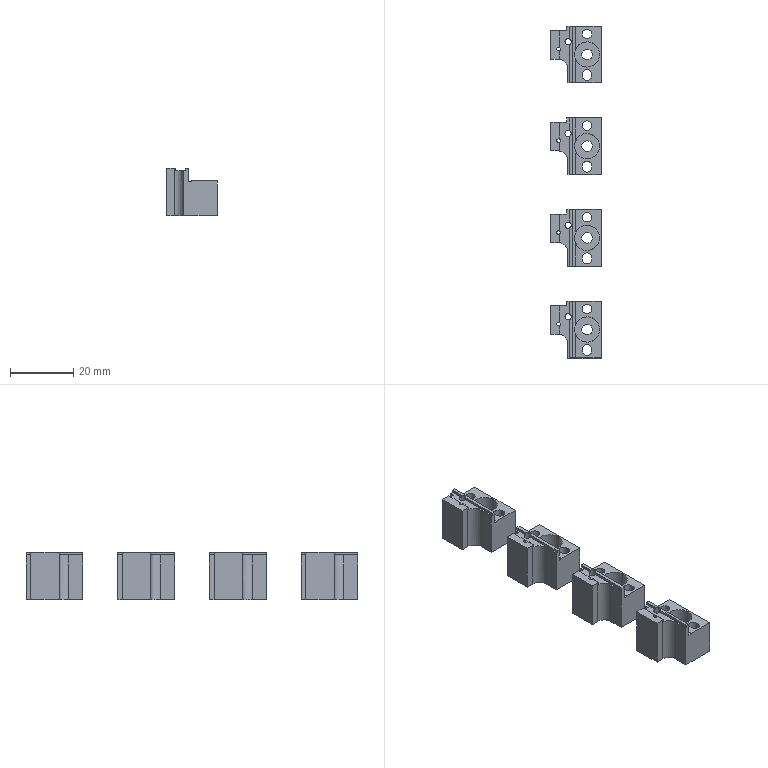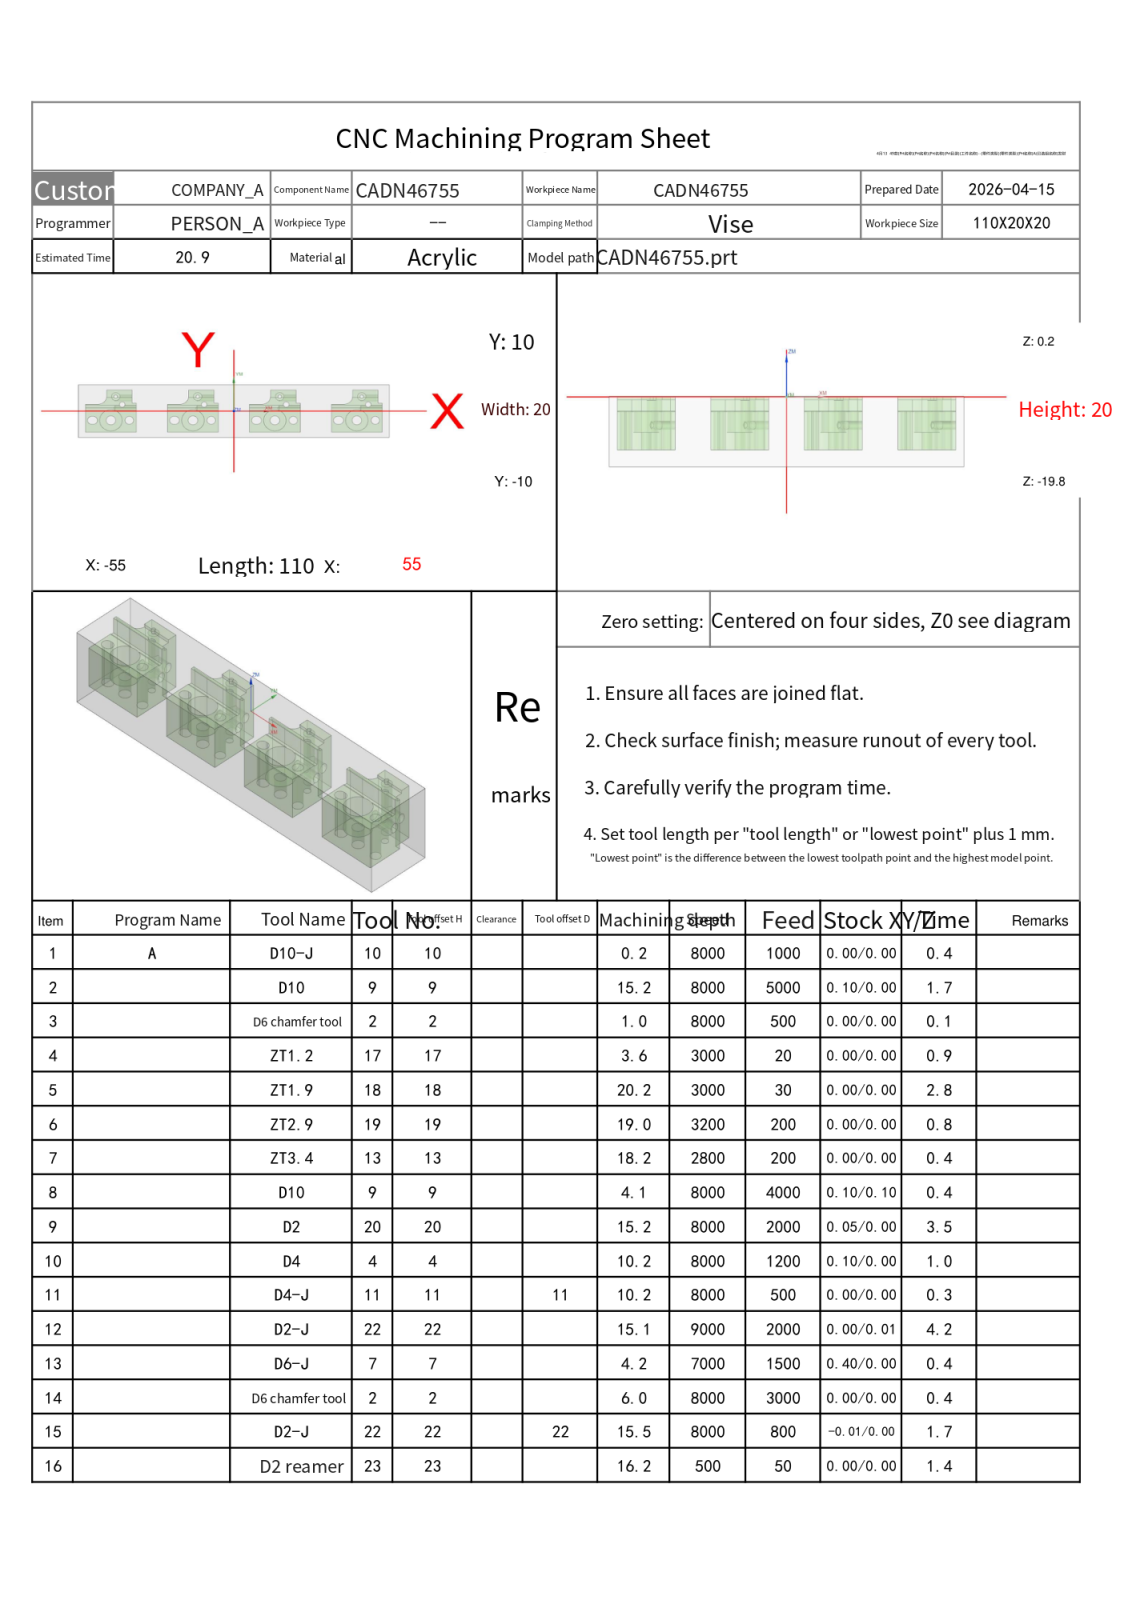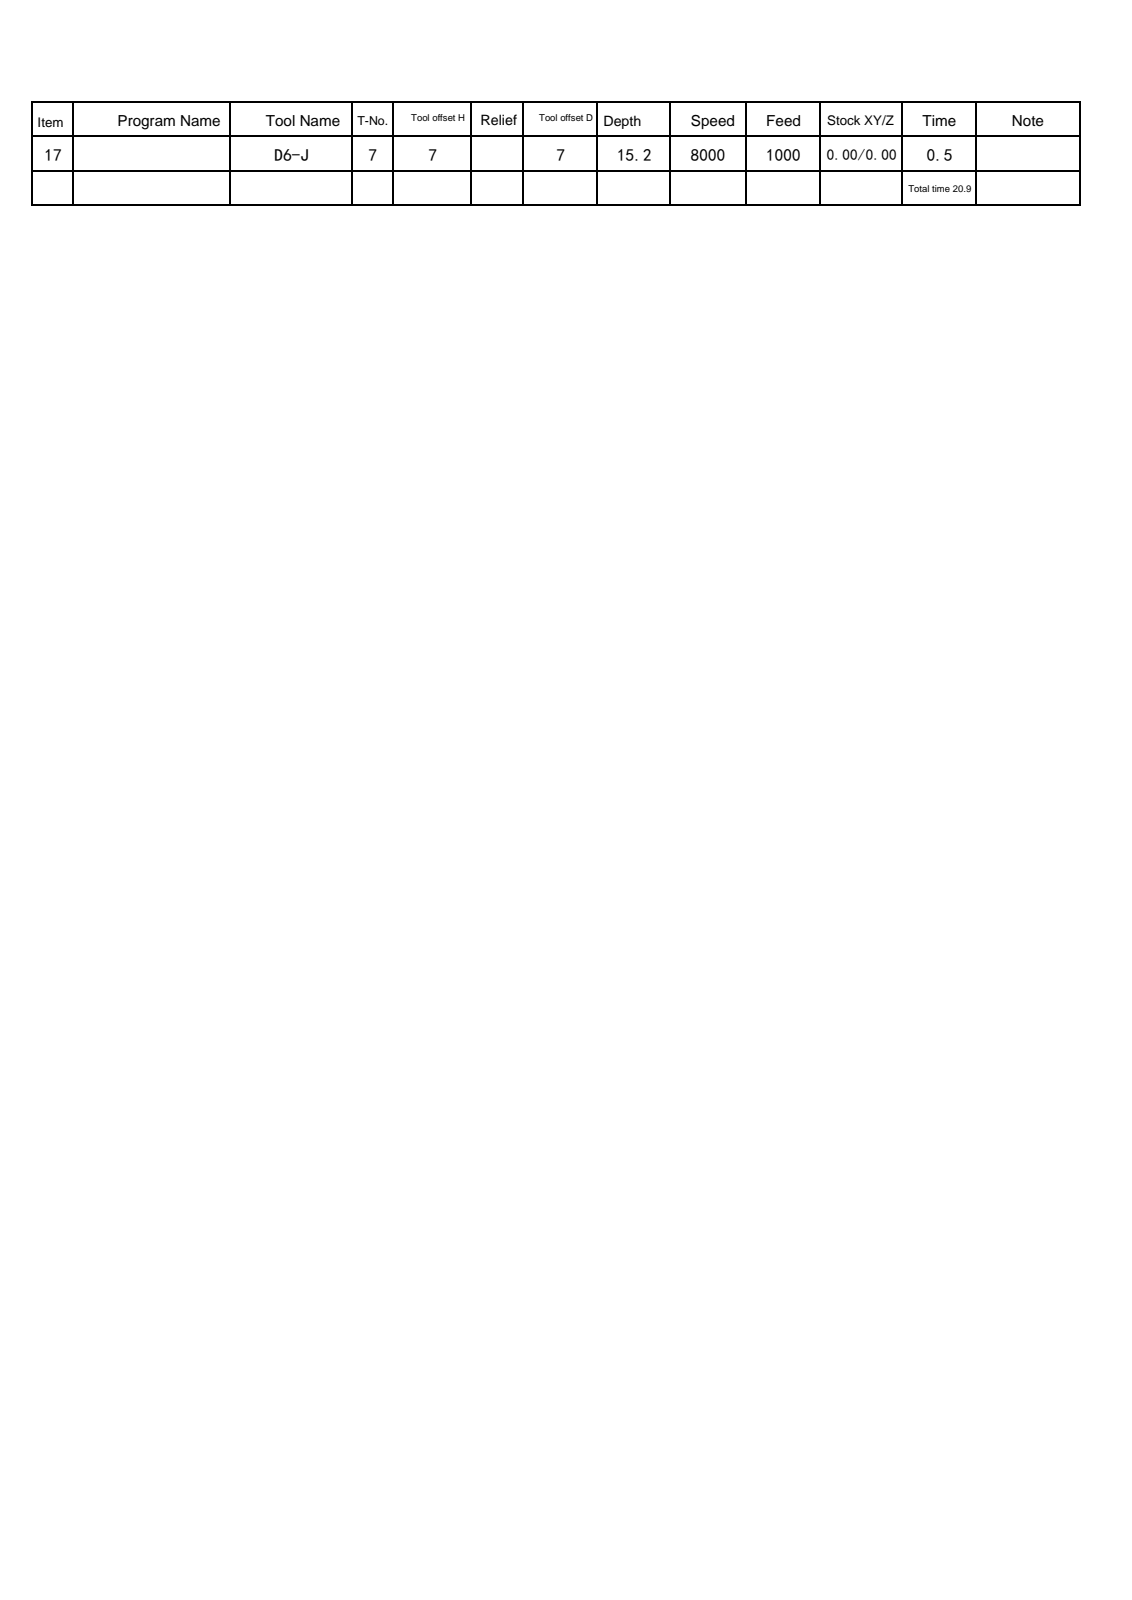NC program | NX | posted by the shop | part box 16 x 105 x 15 mm
Lines 1 to 1402 of 25120, first 1314 of 1400 lines:
%
O0001
(Machine time: 24.18 MIN)
(===Total Tool:13===)
(T10=D10-J  D=10.  R=0.   D-  H10 Z=-0.   )
(T9=D10     D=10.  R=0.   D-  H09 Z=-15.  )
(T2=D6 chamfer tool   D=6.   R=0.   D-  H02 Z=-5.8  )
(T17=ZT1.2  D=1.2  DR_a=118 D-  H17 Z=-3.36 )
(T18=ZT1.9  D=1.9  DR_a=120 D-  H18 Z=-20.  )
(T19=ZT2.9  D=2.9  DR_a=120 D-  H19 Z=-18.84)
(T13=ZT3.4  D=3.4  DR_a=118 D-  H13 Z=-18.02)
(T20=D2     D=2.   R=0.   D-  H20 Z=-15.  )
(T4=D4      D=4.   R=0.   D-  H04 Z=-10.  )
(T11=D4-J   D=4.   R=0.   D11 H11 Z=-10.  )
(T22=D2-J   D=2.   R=0.   D-  H22 Z=-15.3 )
(T7=D6-J    D=6.   R=0.   D-  H07 Z=-15.  )
(T23=D2 reamer   D=1.95 DR_a=180 D23 H23 Z=-16.  )
G80 G90 G17 G49 G40
G91 G28 Z0
M01
N1 T10 M06
(D10-J  D=10. R=0. H=10 ce=0.00 di=0.00)
G00 G90 G54 X-62.5 Y6.5 M03 S8000
G43 H10 Z20.
M08
Z2.
G01 Z0.0 F1000.
X-57.5
X57.5
Y0.0
X-57.5
Y-6.5
X57.5
X62.5
Z2.
G00 Z20.
G91 G28 Z0.0
M05
M09
G91 G28 Z0.0
M01
N2 T09 M06
(D10  D=10. R=0. H=09 ce=0.10 di=0.00)
G00 G90 G54 X43.5 Y-13.1 M03 S8000
G43 H09 Z20.
M08
Z.5
G01 X34.5 Z.428 F5000.
G02 X29.4 Y-8. Z.364 I0.0 J5.1
G01 Y2.6 Z.279
G02 X34.5 Y7.7 Z.215 I5.1 J0.0
G01 X36.9 Z.195
Y8. Z.193
G02 X42. Y13.1 Z.129 I5.1 J0.0
G01 X51. Z.057
G02 X56.1 Y8. Z-.007 I0.0 J-5.1
G01 Y6.612 Z-.018
G02 X57.6 Y3. Z-.051 I-3.6 J-3.612
G01 Y-8. Z-.139
G02 X52.5 Y-13.1 Z-.203 I-5.1 J0.0
G01 X34.5 Z-.347
G02 X29.4 Y-8. Z-.411 I0.0 J5.1
G01 Y2.6 Z-.496
G02 X34.5 Y7.7 Z-.56 I5.1 J0.0
G01 X36.9 Z-.58
Y8. Z-.582
G02 X42. Y13.1 Z-.646 I5.1 J0.0
G01 X51. Z-.718
G02 X56.1 Y8. Z-.782 I0.0 J-5.1
G01 Y6.612 Z-.793
G02 X57.6 Y3. Z-.826 I-3.6 J-3.612
G01 Y-8. Z-.914
G02 X52.5 Y-13.1 Z-.978 I-5.1 J0.0
G01 X34.5 Z-1.122
G02 X29.4 Y-8. Z-1.186 I0.0 J5.1
G01 Y2.6 Z-1.271
G02 X34.5 Y7.7 Z-1.335 I5.1 J0.0
G01 X36.9 Z-1.355
Y8. Z-1.357
G02 X42. Y13.1 Z-1.421 I5.1 J0.0
G01 X51. Z-1.493
G02 X56.1 Y8. Z-1.557 I0.0 J-5.1
G01 Y6.612 Z-1.568
G02 X57.6 Y3. Z-1.601 I-3.6 J-3.612
G01 Y-8. Z-1.689
G02 X52.5 Y-13.1 Z-1.753 I-5.1 J0.0
G01 X34.5 Z-1.897
G02 X29.4 Y-8. Z-1.961 I0.0 J5.1
G01 Y2.6 Z-2.046
G02 X34.5 Y7.7 Z-2.11 I5.1 J0.0
G01 X36.9 Z-2.13
Y8. Z-2.132
G02 X42. Y13.1 Z-2.196 I5.1 J0.0
G01 X51. Z-2.268
G02 X56.1 Y8. Z-2.332 I0.0 J-5.1
G01 Y6.612 Z-2.343
G02 X57.6 Y3. Z-2.376 I-3.6 J-3.612
G01 Y-8. Z-2.464
G02 X52.5 Y-13.1 Z-2.528 I-5.1 J0.0
G01 X34.5 Z-2.672
G02 X29.4 Y-8. Z-2.736 I0.0 J5.1
G01 Y2.6 Z-2.821
G02 X34.5 Y7.7 Z-2.885 I5.1 J0.0
G01 X36.9 Z-2.905
Y8. Z-2.907
G02 X42. Y13.1 Z-2.971 I5.1 J0.0
G01 X51. Z-3.043
G02 X56.1 Y8. Z-3.107 I0.0 J-5.1
G01 Y6.612 Z-3.118
G02 X57.6 Y3. Z-3.151 I-3.6 J-3.612
G01 Y-8. Z-3.239
G02 X52.5 Y-13.1 Z-3.303 I-5.1 J0.0
G01 X34.5 Z-3.447
G02 X29.4 Y-8. Z-3.511 I0.0 J5.1
G01 Y2.6 Z-3.596
G02 X34.5 Y7.7 Z-3.66 I5.1 J0.0
G01 X36.9 Z-3.68
Y8. Z-3.682
G02 X42. Y13.1 Z-3.746 I5.1 J0.0
G01 X51. Z-3.818
G02 X56.1 Y8. Z-3.882 I0.0 J-5.1
G01 Y6.612 Z-3.893
G02 X57.6 Y3. Z-3.926 I-3.6 J-3.612
G01 Y-8. Z-4.014
G02 X52.5 Y-13.1 Z-4.078 I-5.1 J0.0
G01 X34.5 Z-4.222
G02 X29.4 Y-8. Z-4.286 I0.0 J5.1
G01 Y2.6 Z-4.371
G02 X34.5 Y7.7 Z-4.435 I5.1 J0.0
G01 X36.9 Z-4.455
Y8. Z-4.457
G02 X42. Y13.1 Z-4.521 I5.1 J0.0
G01 X51. Z-4.593
G02 X56.1 Y8. Z-4.657 I0.0 J-5.1
G01 Y6.612 Z-4.668
G02 X57.6 Y3. Z-4.701 I-3.6 J-3.612
G01 Y-8. Z-4.789
G02 X52.5 Y-13.1 Z-4.853 I-5.1 J0.0
G01 X34.5 Z-4.997
G02 X29.4 Y-8. Z-5.061 I0.0 J5.1
G01 Y2.6 Z-5.146
G02 X34.5 Y7.7 Z-5.21 I5.1 J0.0
G01 X36.9 Z-5.23
Y8. Z-5.232
G02 X42. Y13.1 Z-5.296 I5.1 J0.0
G01 X51. Z-5.368
G02 X56.1 Y8. Z-5.432 I0.0 J-5.1
G01 Y6.612 Z-5.443
G02 X57.6 Y3. Z-5.476 I-3.6 J-3.612
G01 Y-8. Z-5.564
G02 X52.5 Y-13.1 Z-5.628 I-5.1 J0.0
G01 X34.5 Z-5.772
G02 X29.4 Y-8. Z-5.836 I0.0 J5.1
G01 Y2.6 Z-5.921
G02 X34.5 Y7.7 Z-5.985 I5.1 J0.0
G01 X36.9 Z-6.005
Y8. Z-6.007
G02 X42. Y13.1 Z-6.071 I5.1 J0.0
G01 X51. Z-6.143
G02 X56.1 Y8. Z-6.207 I0.0 J-5.1
G01 Y6.612 Z-6.218
G02 X57.6 Y3. Z-6.251 I-3.6 J-3.612
G01 Y-8. Z-6.339
G02 X52.5 Y-13.1 Z-6.403 I-5.1 J0.0
G01 X34.5 Z-6.547
G02 X29.4 Y-8. Z-6.611 I0.0 J5.1
G01 Y2.6 Z-6.696
G02 X34.5 Y7.7 Z-6.76 I5.1 J0.0
G01 X36.9 Z-6.78
Y8. Z-6.782
G02 X42. Y13.1 Z-6.846 I5.1 J0.0
G01 X51. Z-6.918
G02 X56.1 Y8. Z-6.982 I0.0 J-5.1
G01 Y6.612 Z-6.993
G02 X57.6 Y3. Z-7.026 I-3.6 J-3.612
G01 Y-8. Z-7.114
G02 X52.5 Y-13.1 Z-7.178 I-5.1 J0.0
G01 X34.5 Z-7.322
G02 X29.4 Y-8. Z-7.386 I0.0 J5.1
G01 Y2.6 Z-7.471
G02 X34.5 Y7.7 Z-7.535 I5.1 J0.0
G01 X36.9 Z-7.555
Y8. Z-7.557
G02 X42. Y13.1 Z-7.621 I5.1 J0.0
G01 X51. Z-7.693
G02 X56.1 Y8. Z-7.757 I0.0 J-5.1
G01 Y6.612 Z-7.768
G02 X57.6 Y3. Z-7.801 I-3.6 J-3.612
G01 Y-8. Z-7.889
G02 X52.5 Y-13.1 Z-7.953 I-5.1 J0.0
G01 X34.5 Z-8.097
G02 X29.4 Y-8. Z-8.161 I0.0 J5.1
G01 Y2.6 Z-8.246
G02 X34.5 Y7.7 Z-8.31 I5.1 J0.0
G01 X36.9 Z-8.33
Y8. Z-8.332
G02 X42. Y13.1 Z-8.396 I5.1 J0.0
G01 X51. Z-8.468
G02 X56.1 Y8. Z-8.532 I0.0 J-5.1
G01 Y6.612 Z-8.543
G02 X57.6 Y3. Z-8.576 I-3.6 J-3.612
G01 Y-8. Z-8.664
G02 X52.5 Y-13.1 Z-8.728 I-5.1 J0.0
G01 X34.5 Z-8.872
G02 X29.4 Y-8. Z-8.936 I0.0 J5.1
G01 Y2.6 Z-9.021
G02 X34.5 Y7.7 Z-9.085 I5.1 J0.0
G01 X36.9 Z-9.105
Y8. Z-9.107
G02 X42. Y13.1 Z-9.171 I5.1 J0.0
G01 X51. Z-9.243
G02 X56.1 Y8. Z-9.307 I0.0 J-5.1
G01 Y6.612 Z-9.318
G02 X57.6 Y3. Z-9.351 I-3.6 J-3.612
G01 Y-8. Z-9.439
G02 X52.5 Y-13.1 Z-9.503 I-5.1 J0.0
G01 X34.5 Z-9.647
G02 X29.4 Y-8. Z-9.711 I0.0 J5.1
G01 Y2.6 Z-9.796
G02 X34.5 Y7.7 Z-9.86 I5.1 J0.0
G01 X36.9 Z-9.88
Y8. Z-9.882
G02 X42. Y13.1 Z-9.946 I5.1 J0.0
G01 X51. Z-10.018
G02 X56.1 Y8. Z-10.082 I0.0 J-5.1
G01 Y6.612 Z-10.093
G02 X57.6 Y3. Z-10.126 I-3.6 J-3.612
G01 Y-8. Z-10.214
G02 X52.5 Y-13.1 Z-10.278 I-5.1 J0.0
G01 X34.5 Z-10.422
G02 X29.4 Y-8. Z-10.486 I0.0 J5.1
G01 Y2.6 Z-10.571
G02 X34.5 Y7.7 Z-10.635 I5.1 J0.0
G01 X36.9 Z-10.655
Y8. Z-10.657
G02 X42. Y13.1 Z-10.721 I5.1 J0.0
G01 X51. Z-10.793
G02 X56.1 Y8. Z-10.857 I0.0 J-5.1
G01 Y6.612 Z-10.868
G02 X57.6 Y3. Z-10.901 I-3.6 J-3.612
G01 Y-8. Z-10.989
G02 X52.5 Y-13.1 Z-11.053 I-5.1 J0.0
G01 X34.5 Z-11.197
G02 X29.4 Y-8. Z-11.261 I0.0 J5.1
G01 Y2.6 Z-11.346
G02 X34.5 Y7.7 Z-11.41 I5.1 J0.0
G01 X36.9 Z-11.43
Y8. Z-11.432
G02 X42. Y13.1 Z-11.496 I5.1 J0.0
G01 X51. Z-11.568
G02 X56.1 Y8. Z-11.632 I0.0 J-5.1
G01 Y6.612 Z-11.643
G02 X57.6 Y3. Z-11.676 I-3.6 J-3.612
G01 Y-8. Z-11.764
G02 X52.5 Y-13.1 Z-11.828 I-5.1 J0.0
G01 X34.5 Z-11.972
G02 X29.4 Y-8. Z-12.036 I0.0 J5.1
G01 Y2.6 Z-12.121
G02 X34.5 Y7.7 Z-12.185 I5.1 J0.0
G01 X36.9 Z-12.205
Y8. Z-12.207
G02 X42. Y13.1 Z-12.271 I5.1 J0.0
G01 X51. Z-12.343
G02 X56.1 Y8. Z-12.407 I0.0 J-5.1
G01 Y6.612 Z-12.418
G02 X57.6 Y3. Z-12.451 I-3.6 J-3.612
G01 Y-8. Z-12.539
G02 X52.5 Y-13.1 Z-12.603 I-5.1 J0.0
G01 X34.5 Z-12.747
G02 X29.4 Y-8. Z-12.811 I0.0 J5.1
G01 Y2.6 Z-12.896
G02 X34.5 Y7.7 Z-12.96 I5.1 J0.0
G01 X36.9 Z-12.98
Y8. Z-12.982
G02 X42. Y13.1 Z-13.046 I5.1 J0.0
G01 X51. Z-13.118
G02 X56.1 Y8. Z-13.182 I0.0 J-5.1
G01 Y6.612 Z-13.193
G02 X57.6 Y3. Z-13.226 I-3.6 J-3.612
G01 Y-8. Z-13.314
G02 X52.5 Y-13.1 Z-13.378 I-5.1 J0.0
G01 X34.5 Z-13.522
G02 X29.4 Y-8. Z-13.586 I0.0 J5.1
G01 Y2.6 Z-13.671
G02 X34.5 Y7.7 Z-13.735 I5.1 J0.0
G01 X36.9 Z-13.755
Y8. Z-13.757
G02 X42. Y13.1 Z-13.821 I5.1 J0.0
G01 X51. Z-13.893
G02 X56.1 Y8. Z-13.957 I0.0 J-5.1
G01 Y6.612 Z-13.968
G02 X57.6 Y3. Z-14.001 I-3.6 J-3.612
G01 Y-8. Z-14.089
G02 X52.5 Y-13.1 Z-14.153 I-5.1 J0.0
G01 X34.5 Z-14.297
G02 X29.4 Y-8. Z-14.361 I0.0 J5.1
G01 Y2.6 Z-14.446
G02 X34.5 Y7.7 Z-14.51 I5.1 J0.0
G01 X36.9 Z-14.53
Y8. Z-14.532
G02 X42. Y13.1 Z-14.596 I5.1 J0.0
G01 X51. Z-14.668
G02 X56.1 Y8. Z-14.732 I0.0 J-5.1
G01 Y6.612 Z-14.743
G02 X57.6 Y3. Z-14.776 I-3.6 J-3.612
G01 Y-8. Z-14.864
G02 X52.5 Y-13.1 Z-14.928 I-5.1 J0.0
G01 X43.5 Z-15.
X34.5
G02 X29.4 Y-8. I0.0 J5.1
G01 Y2.6
G02 X34.5 Y7.7 I5.1 J0.0
G01 X36.9
Y8.
G02 X42. Y13.1 I5.1 J0.0
G01 X51.
G02 X56.1 Y8. I0.0 J-5.1
G01 Y6.612
G02 X57.6 Y3. I-3.6 J-3.612
G01 Y-8.
G02 X52.5 Y-13.1 I-5.1 J0.0
G01 X43.5
X43.
Z-14.
G00 Z20.
X14.5
Z.5
G01 X5.5 Z.428
G02 X.4 Y-8. Z.364 I0.0 J5.1
G01 Y2.6 Z.279
G02 X5.5 Y7.7 Z.215 I5.1 J0.0
G01 X7.9 Z.195
Y8. Z.193
G02 X13. Y13.1 Z.129 I5.1 J0.0
G01 X22. Z.057
G02 X27.1 Y8. Z-.007 I0.0 J-5.1
G01 Y6.612 Z-.018
G02 X28.6 Y3. Z-.051 I-3.6 J-3.612
G01 Y-8. Z-.139
G02 X23.5 Y-13.1 Z-.203 I-5.1 J0.0
G01 X5.5 Z-.347
G02 X.4 Y-8. Z-.411 I0.0 J5.1
G01 Y2.6 Z-.496
G02 X5.5 Y7.7 Z-.56 I5.1 J0.0
G01 X7.9 Z-.58
Y8. Z-.582
G02 X13. Y13.1 Z-.646 I5.1 J0.0
G01 X22. Z-.718
G02 X27.1 Y8. Z-.782 I0.0 J-5.1
G01 Y6.612 Z-.793
G02 X28.6 Y3. Z-.826 I-3.6 J-3.612
G01 Y-8. Z-.914
G02 X23.5 Y-13.1 Z-.978 I-5.1 J0.0
G01 X5.5 Z-1.122
G02 X.4 Y-8. Z-1.186 I0.0 J5.1
G01 Y2.6 Z-1.271
G02 X5.5 Y7.7 Z-1.335 I5.1 J0.0
G01 X7.9 Z-1.355
Y8. Z-1.357
G02 X13. Y13.1 Z-1.421 I5.1 J0.0
G01 X22. Z-1.493
G02 X27.1 Y8. Z-1.557 I0.0 J-5.1
G01 Y6.612 Z-1.568
G02 X28.6 Y3. Z-1.601 I-3.6 J-3.612
G01 Y-8. Z-1.689
G02 X23.5 Y-13.1 Z-1.753 I-5.1 J0.0
G01 X5.5 Z-1.897
G02 X.4 Y-8. Z-1.961 I0.0 J5.1
G01 Y2.6 Z-2.046
G02 X5.5 Y7.7 Z-2.11 I5.1 J0.0
G01 X7.9 Z-2.13
Y8. Z-2.132
G02 X13. Y13.1 Z-2.196 I5.1 J0.0
G01 X22. Z-2.268
G02 X27.1 Y8. Z-2.332 I0.0 J-5.1
G01 Y6.612 Z-2.343
G02 X28.6 Y3. Z-2.376 I-3.6 J-3.612
G01 Y-8. Z-2.464
G02 X23.5 Y-13.1 Z-2.528 I-5.1 J0.0
G01 X5.5 Z-2.672
G02 X.4 Y-8. Z-2.736 I0.0 J5.1
G01 Y2.6 Z-2.821
G02 X5.5 Y7.7 Z-2.885 I5.1 J0.0
G01 X7.9 Z-2.905
Y8. Z-2.907
G02 X13. Y13.1 Z-2.971 I5.1 J0.0
G01 X22. Z-3.043
G02 X27.1 Y8. Z-3.107 I0.0 J-5.1
G01 Y6.612 Z-3.118
G02 X28.6 Y3. Z-3.151 I-3.6 J-3.612
G01 Y-8. Z-3.239
G02 X23.5 Y-13.1 Z-3.303 I-5.1 J0.0
G01 X5.5 Z-3.447
G02 X.4 Y-8. Z-3.511 I0.0 J5.1
G01 Y2.6 Z-3.596
G02 X5.5 Y7.7 Z-3.66 I5.1 J0.0
G01 X7.9 Z-3.68
Y8. Z-3.682
G02 X13. Y13.1 Z-3.746 I5.1 J0.0
G01 X22. Z-3.818
G02 X27.1 Y8. Z-3.882 I0.0 J-5.1
G01 Y6.612 Z-3.893
G02 X28.6 Y3. Z-3.926 I-3.6 J-3.612
G01 Y-8. Z-4.014
G02 X23.5 Y-13.1 Z-4.078 I-5.1 J0.0
G01 X5.5 Z-4.222
G02 X.4 Y-8. Z-4.286 I0.0 J5.1
G01 Y2.6 Z-4.371
G02 X5.5 Y7.7 Z-4.435 I5.1 J0.0
G01 X7.9 Z-4.455
Y8. Z-4.457
G02 X13. Y13.1 Z-4.521 I5.1 J0.0
G01 X22. Z-4.593
G02 X27.1 Y8. Z-4.657 I0.0 J-5.1
G01 Y6.612 Z-4.668
G02 X28.6 Y3. Z-4.701 I-3.6 J-3.612
G01 Y-8. Z-4.789
G02 X23.5 Y-13.1 Z-4.853 I-5.1 J0.0
G01 X5.5 Z-4.997
G02 X.4 Y-8. Z-5.061 I0.0 J5.1
G01 Y2.6 Z-5.146
G02 X5.5 Y7.7 Z-5.21 I5.1 J0.0
G01 X7.9 Z-5.23
Y8. Z-5.232
G02 X13. Y13.1 Z-5.296 I5.1 J0.0
G01 X22. Z-5.368
G02 X27.1 Y8. Z-5.432 I0.0 J-5.1
G01 Y6.612 Z-5.443
G02 X28.6 Y3. Z-5.476 I-3.6 J-3.612
G01 Y-8. Z-5.564
G02 X23.5 Y-13.1 Z-5.628 I-5.1 J0.0
G01 X5.5 Z-5.772
G02 X.4 Y-8. Z-5.836 I0.0 J5.1
G01 Y2.6 Z-5.921
G02 X5.5 Y7.7 Z-5.985 I5.1 J0.0
G01 X7.9 Z-6.005
Y8. Z-6.007
G02 X13. Y13.1 Z-6.071 I5.1 J0.0
G01 X22. Z-6.143
G02 X27.1 Y8. Z-6.207 I0.0 J-5.1
G01 Y6.612 Z-6.218
G02 X28.6 Y3. Z-6.251 I-3.6 J-3.612
G01 Y-8. Z-6.339
G02 X23.5 Y-13.1 Z-6.403 I-5.1 J0.0
G01 X5.5 Z-6.547
G02 X.4 Y-8. Z-6.611 I0.0 J5.1
G01 Y2.6 Z-6.696
G02 X5.5 Y7.7 Z-6.76 I5.1 J0.0
G01 X7.9 Z-6.78
Y8. Z-6.782
G02 X13. Y13.1 Z-6.846 I5.1 J0.0
G01 X22. Z-6.918
G02 X27.1 Y8. Z-6.982 I0.0 J-5.1
G01 Y6.612 Z-6.993
G02 X28.6 Y3. Z-7.026 I-3.6 J-3.612
G01 Y-8. Z-7.114
G02 X23.5 Y-13.1 Z-7.178 I-5.1 J0.0
G01 X5.5 Z-7.322
G02 X.4 Y-8. Z-7.386 I0.0 J5.1
G01 Y2.6 Z-7.471
G02 X5.5 Y7.7 Z-7.535 I5.1 J0.0
G01 X7.9 Z-7.555
Y8. Z-7.557
G02 X13. Y13.1 Z-7.621 I5.1 J0.0
G01 X22. Z-7.693
G02 X27.1 Y8. Z-7.757 I0.0 J-5.1
G01 Y6.612 Z-7.768
G02 X28.6 Y3. Z-7.801 I-3.6 J-3.612
G01 Y-8. Z-7.889
G02 X23.5 Y-13.1 Z-7.953 I-5.1 J0.0
G01 X5.5 Z-8.097
G02 X.4 Y-8. Z-8.161 I0.0 J5.1
G01 Y2.6 Z-8.246
G02 X5.5 Y7.7 Z-8.31 I5.1 J0.0
G01 X7.9 Z-8.33
Y8. Z-8.332
G02 X13. Y13.1 Z-8.396 I5.1 J0.0
G01 X22. Z-8.468
G02 X27.1 Y8. Z-8.532 I0.0 J-5.1
G01 Y6.612 Z-8.543
G02 X28.6 Y3. Z-8.576 I-3.6 J-3.612
G01 Y-8. Z-8.664
G02 X23.5 Y-13.1 Z-8.728 I-5.1 J0.0
G01 X5.5 Z-8.872
G02 X.4 Y-8. Z-8.936 I0.0 J5.1
G01 Y2.6 Z-9.021
G02 X5.5 Y7.7 Z-9.085 I5.1 J0.0
G01 X7.9 Z-9.105
Y8. Z-9.107
G02 X13. Y13.1 Z-9.171 I5.1 J0.0
G01 X22. Z-9.243
G02 X27.1 Y8. Z-9.307 I0.0 J-5.1
G01 Y6.612 Z-9.318
G02 X28.6 Y3. Z-9.351 I-3.6 J-3.612
G01 Y-8. Z-9.439
G02 X23.5 Y-13.1 Z-9.503 I-5.1 J0.0
G01 X5.5 Z-9.647
G02 X.4 Y-8. Z-9.711 I0.0 J5.1
G01 Y2.6 Z-9.796
G02 X5.5 Y7.7 Z-9.86 I5.1 J0.0
G01 X7.9 Z-9.88
Y8. Z-9.882
G02 X13. Y13.1 Z-9.946 I5.1 J0.0
G01 X22. Z-10.018
G02 X27.1 Y8. Z-10.082 I0.0 J-5.1
G01 Y6.612 Z-10.093
G02 X28.6 Y3. Z-10.126 I-3.6 J-3.612
G01 Y-8. Z-10.214
G02 X23.5 Y-13.1 Z-10.278 I-5.1 J0.0
G01 X5.5 Z-10.422
G02 X.4 Y-8. Z-10.486 I0.0 J5.1
G01 Y2.6 Z-10.571
G02 X5.5 Y7.7 Z-10.635 I5.1 J0.0
G01 X7.9 Z-10.655
Y8. Z-10.657
G02 X13. Y13.1 Z-10.721 I5.1 J0.0
G01 X22. Z-10.793
G02 X27.1 Y8. Z-10.857 I0.0 J-5.1
G01 Y6.612 Z-10.868
G02 X28.6 Y3. Z-10.901 I-3.6 J-3.612
G01 Y-8. Z-10.989
G02 X23.5 Y-13.1 Z-11.053 I-5.1 J0.0
G01 X5.5 Z-11.197
G02 X.4 Y-8. Z-11.261 I0.0 J5.1
G01 Y2.6 Z-11.346
G02 X5.5 Y7.7 Z-11.41 I5.1 J0.0
G01 X7.9 Z-11.43
Y8. Z-11.432
G02 X13. Y13.1 Z-11.496 I5.1 J0.0
G01 X22. Z-11.568
G02 X27.1 Y8. Z-11.632 I0.0 J-5.1
G01 Y6.612 Z-11.643
G02 X28.6 Y3. Z-11.676 I-3.6 J-3.612
G01 Y-8. Z-11.764
G02 X23.5 Y-13.1 Z-11.828 I-5.1 J0.0
G01 X5.5 Z-11.972
G02 X.4 Y-8. Z-12.036 I0.0 J5.1
G01 Y2.6 Z-12.121
G02 X5.5 Y7.7 Z-12.185 I5.1 J0.0
G01 X7.9 Z-12.205
Y8. Z-12.207
G02 X13. Y13.1 Z-12.271 I5.1 J0.0
G01 X22. Z-12.343
G02 X27.1 Y8. Z-12.407 I0.0 J-5.1
G01 Y6.612 Z-12.418
G02 X28.6 Y3. Z-12.451 I-3.6 J-3.612
G01 Y-8. Z-12.539
G02 X23.5 Y-13.1 Z-12.603 I-5.1 J0.0
G01 X5.5 Z-12.747
G02 X.4 Y-8. Z-12.811 I0.0 J5.1
G01 Y2.6 Z-12.896
G02 X5.5 Y7.7 Z-12.96 I5.1 J0.0
G01 X7.9 Z-12.98
Y8. Z-12.982
G02 X13. Y13.1 Z-13.046 I5.1 J0.0
G01 X22. Z-13.118
G02 X27.1 Y8. Z-13.182 I0.0 J-5.1
G01 Y6.612 Z-13.193
G02 X28.6 Y3. Z-13.226 I-3.6 J-3.612
G01 Y-8. Z-13.314
G02 X23.5 Y-13.1 Z-13.378 I-5.1 J0.0
G01 X5.5 Z-13.522
G02 X.4 Y-8. Z-13.586 I0.0 J5.1
G01 Y2.6 Z-13.671
G02 X5.5 Y7.7 Z-13.735 I5.1 J0.0
G01 X7.9 Z-13.755
Y8. Z-13.757
G02 X13. Y13.1 Z-13.821 I5.1 J0.0
G01 X22. Z-13.893
G02 X27.1 Y8. Z-13.957 I0.0 J-5.1
G01 Y6.612 Z-13.968
G02 X28.6 Y3. Z-14.001 I-3.6 J-3.612
G01 Y-8. Z-14.089
G02 X23.5 Y-13.1 Z-14.153 I-5.1 J0.0
G01 X5.5 Z-14.297
G02 X.4 Y-8. Z-14.361 I0.0 J5.1
G01 Y2.6 Z-14.446
G02 X5.5 Y7.7 Z-14.51 I5.1 J0.0
G01 X7.9 Z-14.53
Y8. Z-14.532
G02 X13. Y13.1 Z-14.596 I5.1 J0.0
G01 X22. Z-14.668
G02 X27.1 Y8. Z-14.732 I0.0 J-5.1
G01 Y6.612 Z-14.743
G02 X28.6 Y3. Z-14.776 I-3.6 J-3.612
G01 Y-8. Z-14.864
G02 X23.5 Y-13.1 Z-14.928 I-5.1 J0.0
G01 X14.5 Z-15.
X5.5
G02 X.4 Y-8. I0.0 J5.1
G01 Y2.6
G02 X5.5 Y7.7 I5.1 J0.0
G01 X7.9
Y8.
G02 X13. Y13.1 I5.1 J0.0
G01 X22.
G02 X27.1 Y8. I0.0 J-5.1
G01 Y6.612
G02 X28.6 Y3. I-3.6 J-3.612
G01 Y-8.
G02 X23.5 Y-13.1 I-5.1 J0.0
G01 X14.5
X14.
Z-14.
G00 Z20.
X-14.5
Z.5
G01 X-23.5 Z.428
G02 X-28.6 Y-8. Z.364 I0.0 J5.1
G01 Y2.6 Z.279
G02 X-23.5 Y7.7 Z.215 I5.1 J0.0
G01 X-21.1 Z.195
Y8. Z.193
G02 X-16. Y13.1 Z.129 I5.1 J0.0
G01 X-7. Z.057
G02 X-1.9 Y8. Z-.007 I0.0 J-5.1
G01 Y6.612 Z-.018
G02 X-.4 Y3. Z-.051 I-3.6 J-3.612
G01 Y-8. Z-.139
G02 X-5.5 Y-13.1 Z-.203 I-5.1 J0.0
G01 X-23.5 Z-.347
G02 X-28.6 Y-8. Z-.411 I0.0 J5.1
G01 Y2.6 Z-.496
G02 X-23.5 Y7.7 Z-.56 I5.1 J0.0
G01 X-21.1 Z-.58
Y8. Z-.582
G02 X-16. Y13.1 Z-.646 I5.1 J0.0
G01 X-7. Z-.718
G02 X-1.9 Y8. Z-.782 I0.0 J-5.1
G01 Y6.612 Z-.793
G02 X-.4 Y3. Z-.826 I-3.6 J-3.612
G01 Y-8. Z-.914
G02 X-5.5 Y-13.1 Z-.978 I-5.1 J0.0
G01 X-23.5 Z-1.122
G02 X-28.6 Y-8. Z-1.186 I0.0 J5.1
G01 Y2.6 Z-1.271
G02 X-23.5 Y7.7 Z-1.335 I5.1 J0.0
G01 X-21.1 Z-1.355
Y8. Z-1.357
G02 X-16. Y13.1 Z-1.421 I5.1 J0.0
G01 X-7. Z-1.493
G02 X-1.9 Y8. Z-1.557 I0.0 J-5.1
G01 Y6.612 Z-1.568
G02 X-.4 Y3. Z-1.601 I-3.6 J-3.612
G01 Y-8. Z-1.689
G02 X-5.5 Y-13.1 Z-1.753 I-5.1 J0.0
G01 X-23.5 Z-1.897
G02 X-28.6 Y-8. Z-1.961 I0.0 J5.1
G01 Y2.6 Z-2.046
G02 X-23.5 Y7.7 Z-2.11 I5.1 J0.0
G01 X-21.1 Z-2.13
Y8. Z-2.132
G02 X-16. Y13.1 Z-2.196 I5.1 J0.0
G01 X-7. Z-2.268
G02 X-1.9 Y8. Z-2.332 I0.0 J-5.1
G01 Y6.612 Z-2.343
G02 X-.4 Y3. Z-2.376 I-3.6 J-3.612
G01 Y-8. Z-2.464
G02 X-5.5 Y-13.1 Z-2.528 I-5.1 J0.0
G01 X-23.5 Z-2.672
G02 X-28.6 Y-8. Z-2.736 I0.0 J5.1
G01 Y2.6 Z-2.821
G02 X-23.5 Y7.7 Z-2.885 I5.1 J0.0
G01 X-21.1 Z-2.905
Y8. Z-2.907
G02 X-16. Y13.1 Z-2.971 I5.1 J0.0
G01 X-7. Z-3.043
G02 X-1.9 Y8. Z-3.107 I0.0 J-5.1
G01 Y6.612 Z-3.118
G02 X-.4 Y3. Z-3.151 I-3.6 J-3.612
G01 Y-8. Z-3.239
G02 X-5.5 Y-13.1 Z-3.303 I-5.1 J0.0
G01 X-23.5 Z-3.447
G02 X-28.6 Y-8. Z-3.511 I0.0 J5.1
G01 Y2.6 Z-3.596
G02 X-23.5 Y7.7 Z-3.66 I5.1 J0.0
G01 X-21.1 Z-3.68
Y8. Z-3.682
G02 X-16. Y13.1 Z-3.746 I5.1 J0.0
G01 X-7. Z-3.818
G02 X-1.9 Y8. Z-3.882 I0.0 J-5.1
G01 Y6.612 Z-3.893
G02 X-.4 Y3. Z-3.926 I-3.6 J-3.612
G01 Y-8. Z-4.014
G02 X-5.5 Y-13.1 Z-4.078 I-5.1 J0.0
G01 X-23.5 Z-4.222
G02 X-28.6 Y-8. Z-4.286 I0.0 J5.1
G01 Y2.6 Z-4.371
G02 X-23.5 Y7.7 Z-4.435 I5.1 J0.0
G01 X-21.1 Z-4.455
Y8. Z-4.457
G02 X-16. Y13.1 Z-4.521 I5.1 J0.0
G01 X-7. Z-4.593
G02 X-1.9 Y8. Z-4.657 I0.0 J-5.1
G01 Y6.612 Z-4.668
G02 X-.4 Y3. Z-4.701 I-3.6 J-3.612
G01 Y-8. Z-4.789
G02 X-5.5 Y-13.1 Z-4.853 I-5.1 J0.0
G01 X-23.5 Z-4.997
G02 X-28.6 Y-8. Z-5.061 I0.0 J5.1
G01 Y2.6 Z-5.146
G02 X-23.5 Y7.7 Z-5.21 I5.1 J0.0
G01 X-21.1 Z-5.23
Y8. Z-5.232
G02 X-16. Y13.1 Z-5.296 I5.1 J0.0
G01 X-7. Z-5.368
G02 X-1.9 Y8. Z-5.432 I0.0 J-5.1
G01 Y6.612 Z-5.443
G02 X-.4 Y3. Z-5.476 I-3.6 J-3.612
G01 Y-8. Z-5.564
G02 X-5.5 Y-13.1 Z-5.628 I-5.1 J0.0
G01 X-23.5 Z-5.772
G02 X-28.6 Y-8. Z-5.836 I0.0 J5.1
G01 Y2.6 Z-5.921
G02 X-23.5 Y7.7 Z-5.985 I5.1 J0.0
G01 X-21.1 Z-6.005
Y8. Z-6.007
G02 X-16. Y13.1 Z-6.071 I5.1 J0.0
G01 X-7. Z-6.143
G02 X-1.9 Y8. Z-6.207 I0.0 J-5.1
G01 Y6.612 Z-6.218
G02 X-.4 Y3. Z-6.251 I-3.6 J-3.612
G01 Y-8. Z-6.339
G02 X-5.5 Y-13.1 Z-6.403 I-5.1 J0.0
G01 X-23.5 Z-6.547
G02 X-28.6 Y-8. Z-6.611 I0.0 J5.1
G01 Y2.6 Z-6.696
G02 X-23.5 Y7.7 Z-6.76 I5.1 J0.0
G01 X-21.1 Z-6.78
Y8. Z-6.782
G02 X-16. Y13.1 Z-6.846 I5.1 J0.0
G01 X-7. Z-6.918
G02 X-1.9 Y8. Z-6.982 I0.0 J-5.1
G01 Y6.612 Z-6.993
G02 X-.4 Y3. Z-7.026 I-3.6 J-3.612
G01 Y-8. Z-7.114
G02 X-5.5 Y-13.1 Z-7.178 I-5.1 J0.0
G01 X-23.5 Z-7.322
G02 X-28.6 Y-8. Z-7.386 I0.0 J5.1
G01 Y2.6 Z-7.471
G02 X-23.5 Y7.7 Z-7.535 I5.1 J0.0
G01 X-21.1 Z-7.555
Y8. Z-7.557
G02 X-16. Y13.1 Z-7.621 I5.1 J0.0
G01 X-7. Z-7.693
G02 X-1.9 Y8. Z-7.757 I0.0 J-5.1
G01 Y6.612 Z-7.768
G02 X-.4 Y3. Z-7.801 I-3.6 J-3.612
G01 Y-8. Z-7.889
G02 X-5.5 Y-13.1 Z-7.953 I-5.1 J0.0
G01 X-23.5 Z-8.097
G02 X-28.6 Y-8. Z-8.161 I0.0 J5.1
G01 Y2.6 Z-8.246
G02 X-23.5 Y7.7 Z-8.31 I5.1 J0.0
G01 X-21.1 Z-8.33
Y8. Z-8.332
G02 X-16. Y13.1 Z-8.396 I5.1 J0.0
G01 X-7. Z-8.468
G02 X-1.9 Y8. Z-8.532 I0.0 J-5.1
G01 Y6.612 Z-8.543
G02 X-.4 Y3. Z-8.576 I-3.6 J-3.612
G01 Y-8. Z-8.664
G02 X-5.5 Y-13.1 Z-8.728 I-5.1 J0.0
G01 X-23.5 Z-8.872
G02 X-28.6 Y-8. Z-8.936 I0.0 J5.1
G01 Y2.6 Z-9.021
G02 X-23.5 Y7.7 Z-9.085 I5.1 J0.0
G01 X-21.1 Z-9.105
Y8. Z-9.107
G02 X-16. Y13.1 Z-9.171 I5.1 J0.0
G01 X-7. Z-9.243
G02 X-1.9 Y8. Z-9.307 I0.0 J-5.1
G01 Y6.612 Z-9.318
G02 X-.4 Y3. Z-9.351 I-3.6 J-3.612
G01 Y-8. Z-9.439
G02 X-5.5 Y-13.1 Z-9.503 I-5.1 J0.0
G01 X-23.5 Z-9.647
G02 X-28.6 Y-8. Z-9.711 I0.0 J5.1
G01 Y2.6 Z-9.796
G02 X-23.5 Y7.7 Z-9.86 I5.1 J0.0
G01 X-21.1 Z-9.88
Y8. Z-9.882
G02 X-16. Y13.1 Z-9.946 I5.1 J0.0
G01 X-7. Z-10.018
G02 X-1.9 Y8. Z-10.082 I0.0 J-5.1
G01 Y6.612 Z-10.093
G02 X-.4 Y3. Z-10.126 I-3.6 J-3.612
G01 Y-8. Z-10.214
G02 X-5.5 Y-13.1 Z-10.278 I-5.1 J0.0
G01 X-23.5 Z-10.422
G02 X-28.6 Y-8. Z-10.486 I0.0 J5.1
G01 Y2.6 Z-10.571
G02 X-23.5 Y7.7 Z-10.635 I5.1 J0.0
G01 X-21.1 Z-10.655
Y8. Z-10.657
G02 X-16. Y13.1 Z-10.721 I5.1 J0.0
G01 X-7. Z-10.793
G02 X-1.9 Y8. Z-10.857 I0.0 J-5.1
G01 Y6.612 Z-10.868
G02 X-.4 Y3. Z-10.901 I-3.6 J-3.612
G01 Y-8. Z-10.989
G02 X-5.5 Y-13.1 Z-11.053 I-5.1 J0.0
G01 X-23.5 Z-11.197
G02 X-28.6 Y-8. Z-11.261 I0.0 J5.1
G01 Y2.6 Z-11.346
G02 X-23.5 Y7.7 Z-11.41 I5.1 J0.0
G01 X-21.1 Z-11.43
Y8. Z-11.432
G02 X-16. Y13.1 Z-11.496 I5.1 J0.0
G01 X-7. Z-11.568
G02 X-1.9 Y8. Z-11.632 I0.0 J-5.1
G01 Y6.612 Z-11.643
G02 X-.4 Y3. Z-11.676 I-3.6 J-3.612
G01 Y-8. Z-11.764
G02 X-5.5 Y-13.1 Z-11.828 I-5.1 J0.0
G01 X-23.5 Z-11.972
G02 X-28.6 Y-8. Z-12.036 I0.0 J5.1
G01 Y2.6 Z-12.121
G02 X-23.5 Y7.7 Z-12.185 I5.1 J0.0
G01 X-21.1 Z-12.205
Y8. Z-12.207
G02 X-16. Y13.1 Z-12.271 I5.1 J0.0
G01 X-7. Z-12.343
G02 X-1.9 Y8. Z-12.407 I0.0 J-5.1
G01 Y6.612 Z-12.418
G02 X-.4 Y3. Z-12.451 I-3.6 J-3.612
G01 Y-8. Z-12.539
G02 X-5.5 Y-13.1 Z-12.603 I-5.1 J0.0
G01 X-23.5 Z-12.747
G02 X-28.6 Y-8. Z-12.811 I0.0 J5.1
G01 Y2.6 Z-12.896
G02 X-23.5 Y7.7 Z-12.96 I5.1 J0.0
G01 X-21.1 Z-12.98
Y8. Z-12.982
G02 X-16. Y13.1 Z-13.046 I5.1 J0.0
G01 X-7. Z-13.118
G02 X-1.9 Y8. Z-13.182 I0.0 J-5.1
G01 Y6.612 Z-13.193
G02 X-.4 Y3. Z-13.226 I-3.6 J-3.612
G01 Y-8. Z-13.314
G02 X-5.5 Y-13.1 Z-13.378 I-5.1 J0.0
G01 X-23.5 Z-13.522
G02 X-28.6 Y-8. Z-13.586 I0.0 J5.1
G01 Y2.6 Z-13.671
G02 X-23.5 Y7.7 Z-13.735 I5.1 J0.0
G01 X-21.1 Z-13.755
Y8. Z-13.757
G02 X-16. Y13.1 Z-13.821 I5.1 J0.0
G01 X-7. Z-13.893
G02 X-1.9 Y8. Z-13.957 I0.0 J-5.1
G01 Y6.612 Z-13.968
G02 X-.4 Y3. Z-14.001 I-3.6 J-3.612
G01 Y-8. Z-14.089
G02 X-5.5 Y-13.1 Z-14.153 I-5.1 J0.0
G01 X-23.5 Z-14.297
G02 X-28.6 Y-8. Z-14.361 I0.0 J5.1
G01 Y2.6 Z-14.446
G02 X-23.5 Y7.7 Z-14.51 I5.1 J0.0
G01 X-21.1 Z-14.53
Y8. Z-14.532
G02 X-16. Y13.1 Z-14.596 I5.1 J0.0
G01 X-7. Z-14.668
G02 X-1.9 Y8. Z-14.732 I0.0 J-5.1
G01 Y6.612 Z-14.743
G02 X-.4 Y3. Z-14.776 I-3.6 J-3.612
G01 Y-8. Z-14.864
G02 X-5.5 Y-13.1 Z-14.928 I-5.1 J0.0
G01 X-14.5 Z-15.
X-23.5
G02 X-28.6 Y-8. I0.0 J5.1
G01 Y2.6
G02 X-23.5 Y7.7 I5.1 J0.0
G01 X-21.1
Y8.
G02 X-16. Y13.1 I5.1 J0.0
G01 X-7.
G02 X-1.9 Y8. I0.0 J-5.1
G01 Y6.612
G02 X-.4 Y3. I-3.6 J-3.612
G01 Y-8.
G02 X-5.5 Y-13.1 I-5.1 J0.0
G01 X-14.5
X-15.
Z-14.
G00 Z20.
X-43.5
Z.5
G01 X-52.5 Z.428
G02 X-57.6 Y-8. Z.364 I0.0 J5.1
G01 Y2.6 Z.279
G02 X-52.5 Y7.7 Z.215 I5.1 J0.0
G01 X-50.1 Z.195
Y8. Z.193
G02 X-45. Y13.1 Z.129 I5.1 J0.0
G01 X-36. Z.057
G02 X-30.9 Y8. Z-.007 I0.0 J-5.1
G01 Y6.612 Z-.018
G02 X-29.4 Y3. Z-.051 I-3.6 J-3.612
G01 Y-8. Z-.139
G02 X-34.5 Y-13.1 Z-.203 I-5.1 J0.0
G01 X-52.5 Z-.347
G02 X-57.6 Y-8. Z-.411 I0.0 J5.1
G01 Y2.6 Z-.496
G02 X-52.5 Y7.7 Z-.56 I5.1 J0.0
G01 X-50.1 Z-.58
Y8. Z-.582
G02 X-45. Y13.1 Z-.646 I5.1 J0.0
G01 X-36. Z-.718
G02 X-30.9 Y8. Z-.782 I0.0 J-5.1
G01 Y6.612 Z-.793
G02 X-29.4 Y3. Z-.826 I-3.6 J-3.612
G01 Y-8. Z-.914
G02 X-34.5 Y-13.1 Z-.978 I-5.1 J0.0
G01 X-52.5 Z-1.122
G02 X-57.6 Y-8. Z-1.186 I0.0 J5.1
G01 Y2.6 Z-1.271
G02 X-52.5 Y7.7 Z-1.335 I5.1 J0.0
G01 X-50.1 Z-1.355
Y8. Z-1.357
G02 X-45. Y13.1 Z-1.421 I5.1 J0.0
G01 X-36. Z-1.493
G02 X-30.9 Y8. Z-1.557 I0.0 J-5.1
G01 Y6.612 Z-1.568
G02 X-29.4 Y3. Z-1.601 I-3.6 J-3.612
G01 Y-8. Z-1.689
G02 X-34.5 Y-13.1 Z-1.753 I-5.1 J0.0
G01 X-52.5 Z-1.897
G02 X-57.6 Y-8. Z-1.961 I0.0 J5.1
G01 Y2.6 Z-2.046
G02 X-52.5 Y7.7 Z-2.11 I5.1 J0.0
G01 X-50.1 Z-2.13
Y8. Z-2.132
G02 X-45. Y13.1 Z-2.196 I5.1 J0.0
G01 X-36. Z-2.268
G02 X-30.9 Y8. Z-2.332 I0.0 J-5.1
G01 Y6.612 Z-2.343
G02 X-29.4 Y3. Z-2.376 I-3.6 J-3.612
G01 Y-8. Z-2.464
G02 X-34.5 Y-13.1 Z-2.528 I-5.1 J0.0
G01 X-52.5 Z-2.672
G02 X-57.6 Y-8. Z-2.736 I0.0 J5.1
G01 Y2.6 Z-2.821
G02 X-52.5 Y7.7 Z-2.885 I5.1 J0.0
G01 X-50.1 Z-2.905
Y8. Z-2.907
G02 X-45. Y13.1 Z-2.971 I5.1 J0.0
G01 X-36. Z-3.043
G02 X-30.9 Y8. Z-3.107 I0.0 J-5.1
G01 Y6.612 Z-3.118
G02 X-29.4 Y3. Z-3.151 I-3.6 J-3.612
G01 Y-8. Z-3.239
G02 X-34.5 Y-13.1 Z-3.303 I-5.1 J0.0
G01 X-52.5 Z-3.447
G02 X-57.6 Y-8. Z-3.511 I0.0 J5.1
G01 Y2.6 Z-3.596
G02 X-52.5 Y7.7 Z-3.66 I5.1 J0.0
G01 X-50.1 Z-3.68
Y8. Z-3.682
G02 X-45. Y13.1 Z-3.746 I5.1 J0.0
G01 X-36. Z-3.818
G02 X-30.9 Y8. Z-3.882 I0.0 J-5.1
G01 Y6.612 Z-3.893
G02 X-29.4 Y3. Z-3.926 I-3.6 J-3.612
G01 Y-8. Z-4.014
G02 X-34.5 Y-13.1 Z-4.078 I-5.1 J0.0
G01 X-52.5 Z-4.222
G02 X-57.6 Y-8. Z-4.286 I0.0 J5.1
G01 Y2.6 Z-4.371
G02 X-52.5 Y7.7 Z-4.435 I5.1 J0.0
G01 X-50.1 Z-4.455
Y8. Z-4.457
G02 X-45. Y13.1 Z-4.521 I5.1 J0.0
G01 X-36. Z-4.593
G02 X-30.9 Y8. Z-4.657 I0.0 J-5.1
G01 Y6.612 Z-4.668
G02 X-29.4 Y3. Z-4.701 I-3.6 J-3.612
G01 Y-8. Z-4.789
G02 X-34.5 Y-13.1 Z-4.853 I-5.1 J0.0
G01 X-52.5 Z-4.997
G02 X-57.6 Y-8. Z-5.061 I0.0 J5.1
G01 Y2.6 Z-5.146
G02 X-52.5 Y7.7 Z-5.21 I5.1 J0.0
G01 X-50.1 Z-5.23
Y8. Z-5.232
G02 X-45. Y13.1 Z-5.296 I5.1 J0.0
G01 X-36. Z-5.368
G02 X-30.9 Y8. Z-5.432 I0.0 J-5.1
G01 Y6.612 Z-5.443
G02 X-29.4 Y3. Z-5.476 I-3.6 J-3.612
G01 Y-8. Z-5.564
G02 X-34.5 Y-13.1 Z-5.628 I-5.1 J0.0
G01 X-52.5 Z-5.772
G02 X-57.6 Y-8. Z-5.836 I0.0 J5.1
G01 Y2.6 Z-5.921
G02 X-52.5 Y7.7 Z-5.985 I5.1 J0.0
G01 X-50.1 Z-6.005
Y8. Z-6.007
G02 X-45. Y13.1 Z-6.071 I5.1 J0.0
G01 X-36. Z-6.143
G02 X-30.9 Y8. Z-6.207 I0.0 J-5.1
G01 Y6.612 Z-6.218
G02 X-29.4 Y3. Z-6.251 I-3.6 J-3.612
G01 Y-8. Z-6.339
G02 X-34.5 Y-13.1 Z-6.403 I-5.1 J0.0
G01 X-52.5 Z-6.547
G02 X-57.6 Y-8. Z-6.611 I0.0 J5.1
G01 Y2.6 Z-6.696
G02 X-52.5 Y7.7 Z-6.76 I5.1 J0.0
G01 X-50.1 Z-6.78
Y8. Z-6.782
G02 X-45. Y13.1 Z-6.846 I5.1 J0.0
G01 X-36. Z-6.918
G02 X-30.9 Y8. Z-6.982 I0.0 J-5.1
G01 Y6.612 Z-6.993
G02 X-29.4 Y3. Z-7.026 I-3.6 J-3.612
G01 Y-8. Z-7.114
G02 X-34.5 Y-13.1 Z-7.178 I-5.1 J0.0
G01 X-52.5 Z-7.322
G02 X-57.6 Y-8. Z-7.386 I0.0 J5.1
G01 Y2.6 Z-7.471
G02 X-52.5 Y7.7 Z-7.535 I5.1 J0.0
G01 X-50.1 Z-7.555
Y8. Z-7.557
G02 X-45. Y13.1 Z-7.621 I5.1 J0.0
G01 X-36. Z-7.693
G02 X-30.9 Y8. Z-7.757 I0.0 J-5.1
G01 Y6.612 Z-7.768
G02 X-29.4 Y3. Z-7.801 I-3.6 J-3.612
G01 Y-8. Z-7.889
G02 X-34.5 Y-13.1 Z-7.953 I-5.1 J0.0
G01 X-52.5 Z-8.097
G02 X-57.6 Y-8. Z-8.161 I0.0 J5.1
G01 Y2.6 Z-8.246
G02 X-52.5 Y7.7 Z-8.31 I5.1 J0.0
G01 X-50.1 Z-8.33
Y8. Z-8.332
G02 X-45. Y13.1 Z-8.396 I5.1 J0.0
G01 X-36. Z-8.468
G02 X-30.9 Y8. Z-8.532 I0.0 J-5.1
G01 Y6.612 Z-8.543
G02 X-29.4 Y3. Z-8.576 I-3.6 J-3.612
G01 Y-8. Z-8.664
G02 X-34.5 Y-13.1 Z-8.728 I-5.1 J0.0
G01 X-52.5 Z-8.872
G02 X-57.6 Y-8. Z-8.936 I0.0 J5.1
G01 Y2.6 Z-9.021
G02 X-52.5 Y7.7 Z-9.085 I5.1 J0.0
G01 X-50.1 Z-9.105
Y8. Z-9.107
G02 X-45. Y13.1 Z-9.171 I5.1 J0.0
G01 X-36. Z-9.243
G02 X-30.9 Y8. Z-9.307 I0.0 J-5.1
G01 Y6.612 Z-9.318
G02 X-29.4 Y3. Z-9.351 I-3.6 J-3.612
G01 Y-8. Z-9.439
G02 X-34.5 Y-13.1 Z-9.503 I-5.1 J0.0
G01 X-52.5 Z-9.647
G02 X-57.6 Y-8. Z-9.711 I0.0 J5.1
G01 Y2.6 Z-9.796
G02 X-52.5 Y7.7 Z-9.86 I5.1 J0.0
G01 X-50.1 Z-9.88
Y8. Z-9.882
G02 X-45. Y13.1 Z-9.946 I5.1 J0.0
G01 X-36. Z-10.018
G02 X-30.9 Y8. Z-10.082 I0.0 J-5.1
G01 Y6.612 Z-10.093
G02 X-29.4 Y3. Z-10.126 I-3.6 J-3.612
G01 Y-8. Z-10.214
G02 X-34.5 Y-13.1 Z-10.278 I-5.1 J0.0
G01 X-52.5 Z-10.422
G02 X-57.6 Y-8. Z-10.486 I0.0 J5.1
G01 Y2.6 Z-10.571
G02 X-52.5 Y7.7 Z-10.635 I5.1 J0.0
G01 X-50.1 Z-10.655
Y8. Z-10.657
G02 X-45. Y13.1 Z-10.721 I5.1 J0.0
G01 X-36. Z-10.793
G02 X-30.9 Y8. Z-10.857 I0.0 J-5.1
G01 Y6.612 Z-10.868
G02 X-29.4 Y3. Z-10.901 I-3.6 J-3.612
G01 Y-8. Z-10.989
G02 X-34.5 Y-13.1 Z-11.053 I-5.1 J0.0
G01 X-52.5 Z-11.197
G02 X-57.6 Y-8. Z-11.261 I0.0 J5.1
G01 Y2.6 Z-11.346
G02 X-52.5 Y7.7 Z-11.41 I5.1 J0.0
G01 X-50.1 Z-11.43
Y8. Z-11.432
G02 X-45. Y13.1 Z-11.496 I5.1 J0.0
G01 X-36. Z-11.568
G02 X-30.9 Y8. Z-11.632 I0.0 J-5.1
G01 Y6.612 Z-11.643
G02 X-29.4 Y3. Z-11.676 I-3.6 J-3.612
G01 Y-8. Z-11.764
G02 X-34.5 Y-13.1 Z-11.828 I-5.1 J0.0
G01 X-52.5 Z-11.972
G02 X-57.6 Y-8. Z-12.036 I0.0 J5.1
G01 Y2.6 Z-12.121
G02 X-52.5 Y7.7 Z-12.185 I5.1 J0.0
G01 X-50.1 Z-12.205
Y8. Z-12.207
G02 X-45. Y13.1 Z-12.271 I5.1 J0.0
G01 X-36. Z-12.343
G02 X-30.9 Y8. Z-12.407 I0.0 J-5.1
G01 Y6.612 Z-12.418
G02 X-29.4 Y3. Z-12.451 I-3.6 J-3.612
G01 Y-8. Z-12.539
G02 X-34.5 Y-13.1 Z-12.603 I-5.1 J0.0
G01 X-52.5 Z-12.747
G02 X-57.6 Y-8. Z-12.811 I0.0 J5.1
G01 Y2.6 Z-12.896
G02 X-52.5 Y7.7 Z-12.96 I5.1 J0.0
G01 X-50.1 Z-12.98
Y8. Z-12.982
G02 X-45. Y13.1 Z-13.046 I5.1 J0.0
G01 X-36. Z-13.118
G02 X-30.9 Y8. Z-13.182 I0.0 J-5.1
G01 Y6.612 Z-13.193
G02 X-29.4 Y3. Z-13.226 I-3.6 J-3.612
G01 Y-8. Z-13.314
G02 X-34.5 Y-13.1 Z-13.378 I-5.1 J0.0
G01 X-52.5 Z-13.522
G02 X-57.6 Y-8. Z-13.586 I0.0 J5.1
G01 Y2.6 Z-13.671
G02 X-52.5 Y7.7 Z-13.735 I5.1 J0.0
G01 X-50.1 Z-13.755
Y8. Z-13.757
G02 X-45. Y13.1 Z-13.821 I5.1 J0.0
G01 X-36. Z-13.893
G02 X-30.9 Y8. Z-13.957 I0.0 J-5.1
G01 Y6.612 Z-13.968
G02 X-29.4 Y3. Z-14.001 I-3.6 J-3.612
G01 Y-8. Z-14.089
G02 X-34.5 Y-13.1 Z-14.153 I-5.1 J0.0
G01 X-52.5 Z-14.297
G02 X-57.6 Y-8. Z-14.361 I0.0 J5.1
G01 Y2.6 Z-14.446
G02 X-52.5 Y7.7 Z-14.51 I5.1 J0.0
G01 X-50.1 Z-14.53
Y8. Z-14.532
G02 X-45. Y13.1 Z-14.596 I5.1 J0.0
G01 X-36. Z-14.668
G02 X-30.9 Y8. Z-14.732 I0.0 J-5.1
G01 Y6.612 Z-14.743
G02 X-29.4 Y3. Z-14.776 I-3.6 J-3.612
G01 Y-8. Z-14.864
G02 X-34.5 Y-13.1 Z-14.928 I-5.1 J0.0
G01 X-43.5 Z-15.
X-52.5
G02 X-57.6 Y-8. I0.0 J5.1
G01 Y2.6
G02 X-52.5 Y7.7 I5.1 J0.0
G01 X-50.1
Y8.
G02 X-45. Y13.1 I5.1 J0.0
G01 X-36.
G02 X-30.9 Y8. I0.0 J-5.1
G01 Y6.612
G02 X-29.4 Y3. I-3.6 J-3.612
G01 Y-8.
G02 X-34.5 Y-13.1 I-5.1 J0.0
G01 X-43.5
X-44.
Z-14.
G00 Z20.
G91 G28 Z0.0
M05
M09
G91 G28 Z0.0
M01
N3 T02 M06
(D6 chamfer tool  D=6. R=0. H=02 ce=0.00 di=0.00)
G00 G90 G54 X45.2 Y5.5 M03 S8000
G43 H02 Z20.
M08
G98 G81 X45.2 Y5.5 Z-.8 R1. F500.
X47.5 Y2.5
X50. Y-3.5
X43.5
X21.
X14.5
X18.5 Y2.5
X16.2 Y5.5
X-12.8
X-10.5 Y2.5
X-8. Y-3.5
X-14.5
X-37.
X-43.5
X-39.5 Y2.5
X-41.8 Y5.5
X-49.75 Y-3.5
X-20.75
X8.25
X37.25
G80
G00 Z20.
G91 G28 Z0.0
M05
M09
G91 G28 Z0.0
M01
N4 T17 M06
(ZT1.2 D=1.2 DR_a=118 H=17)
G00 G90 G54 X-41.8 Y5.5 M03 S3000
G43 H17 Z20.
M08
G98 G83 X-41.8 Y5.5 Z-3.361 R1. F20. Q1.5
X-12.8
X16.2
X45.2
G80
G00 Z20.
G91 G28 Z0.0
M05
M09
G91 G28 Z0.0
M01
N5 T18 M06
(ZT1.9 D=1.9 DR_a=120 H=18)
G00 G90 G54 X-39.5 Y2.5 M03 S3000
G43 H18 Z20.
M08
G98 G83 X-39.5 Y2.5 Z-20. R1. F30. Q1.5
X-10.5
X18.5
X47.5
G80
G00 Z20.
G91 G28 Z0.0
M05
M09
G91 G28 Z0.0
M01
N6 T19 M06
(ZT2.9 D=2.9 DR_a=120 H=19)
G00 G90 G54 X-37. Y-3.5 M03 S3200
G43 H19 Z20.
M08
G98 G83 X-37. Y-3.5 Z-18.837 R1. F200. Q2.
X-8.
X21.
X50.
X-49.75
X-20.75
X8.25
X37.25
G80
G00 Z20.
G91 G28 Z0.0
M05
M09
G91 G28 Z0.0
M01
N7 T13 M06
(ZT3.4 D=3.4 DR_a=118 H=13)
G00 G90 G54 X-43.5 Y-3.5 M03 S2800
G43 H13 Z20.
M08
G98 G83 X-43.5 Y-3.5 Z-18.021 R1. F200. Q2.
X-14.5
X14.5
X43.5
G80
G00 Z20.
G91 G28 Z0.0
M05
M09
G91 G28 Z0.0
M01
N8 T09 M06
(D10  D=10. R=0. H=09 ce=0.10 di=0.10)
G00 G90 G54 X-14.5 Y-16. M03 S8000
G43 H09 Z10.2
M08
Z-.08
G01 Z-1.58 F4000.
Y-12.9
X-57.4
Y-3.9
X-29.4
Y5.1
X-28.6
Y-3.9
X-.4
Y5.1
X.4
Y-3.9
X28.6
Y5.1
X29.4
Y-3.9
X57.4
Y-12.9
X-14.5
X-15.
Y-16.
Z-.08
G00 X-14.5
Z-.66
G01 Z-2.16
Y-12.9
X-57.4
Y-3.9
X-29.4
Y5.1
X-28.6
Y-3.9
X-.4
Y5.1
X.4
Y-3.9
X28.6
Y5.1